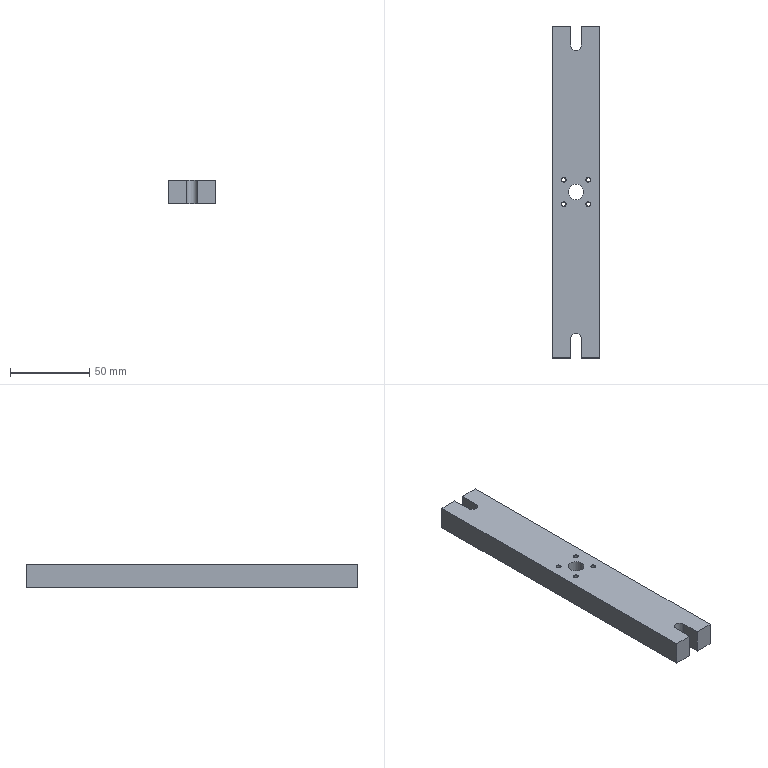Part | STEP file | 1 solid | 27 faces | box 30 x 210 x 15 mm | volume 89928 mm3 | plane 12 | cone 8 | cylinder 7 | commonest cylinder face diameters 2.5 x4 7 x2 10 x1